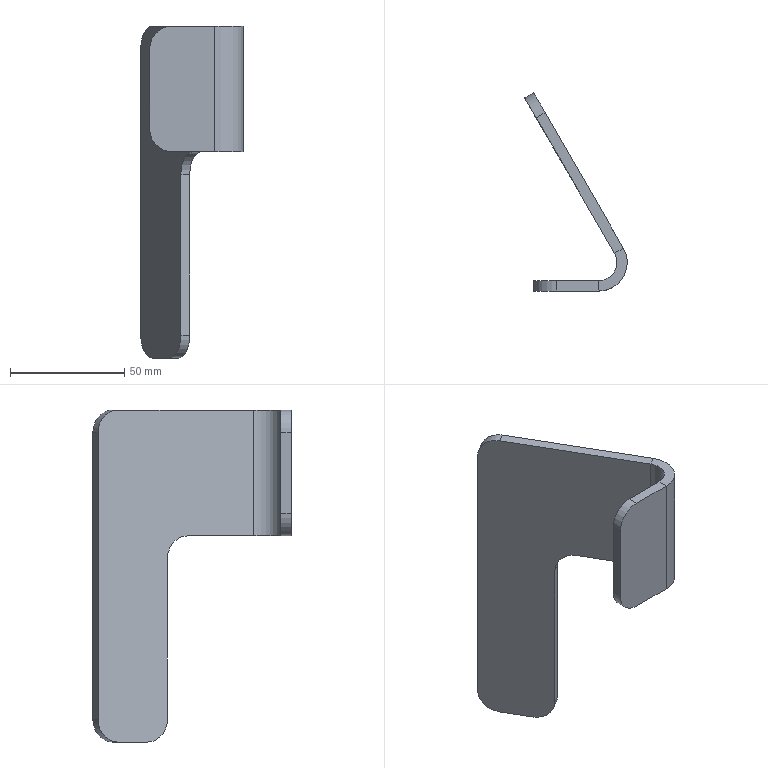Part | SolidWorks | features Fillet 1, FlatPattern 1, ICE 1, SMBaseFlange 1, SheetMetal 1 | 1 solid | 22 faces | box 44.746 x 86.603 x 145 mm | volume 45510 mm3 | plane 14 | cylinder 8 | commonest cylinder face diameters 20 x6 16 x1 25 x1
STEP:
#1=CARTESIAN_POINT('',(-40.,0.,17.5));
#2=VERTEX_POINT('',#1);
#3=CARTESIAN_POINT('',(-21.651,0.,17.5));
#4=VERTEX_POINT('',#3);
#5=CARTESIAN_POINT('',(0.,0.,17.5));
#6=DIRECTION('',(1.,0.,0.));
#7=VECTOR('',#6,1000.);
#8=LINE('',#5,#7);
#9=EDGE_CURVE('',#2,#4,#8,.T.);
#10=ORIENTED_EDGE('',*,*,#9,.F.);
#11=CARTESIAN_POINT('',(-40.,4.5,17.5));
#12=VERTEX_POINT('',#11);
#13=CARTESIAN_POINT('',(-40.,4.5,17.5));
#14=DIRECTION('',(0.,1.,0.));
#15=VECTOR('',#14,1000.);
#16=LINE('',#13,#15);
#17=EDGE_CURVE('',#2,#12,#16,.T.);
#18=ORIENTED_EDGE('',*,*,#17,.T.);
#19=CARTESIAN_POINT('',(-21.651,4.5,17.5));
#20=VERTEX_POINT('',#19);
#21=CARTESIAN_POINT('',(0.,4.5,17.5));
#22=DIRECTION('',(1.,0.,0.));
#23=VECTOR('',#22,1000.);
#24=LINE('',#21,#23);
#25=EDGE_CURVE('',#12,#20,#24,.T.);
#26=ORIENTED_EDGE('',*,*,#25,.T.);
#27=CARTESIAN_POINT('',(-21.651,4.5,17.5));
#28=DIRECTION('',(0.,-1.,0.));
#29=VECTOR('',#28,1000.);
#30=LINE('',#27,#29);
#31=EDGE_CURVE('',#20,#4,#30,.T.);
#32=ORIENTED_EDGE('',*,*,#31,.T.);
#33=EDGE_LOOP('',(#10,#18,#26,#32));
#34=FACE_OUTER_BOUND('',#33,.T.);
#35=CARTESIAN_POINT('',(-67.923,24.293,17.5));
#36=DIRECTION('',(0.,0.,1.));
#37=DIRECTION('',(0.,-1.,0.));
#38=AXIS2_PLACEMENT_3D('',#35,#36,#37);
#39=PLANE('',#38);
#40=ADVANCED_FACE('',(#34),#39,.F.);
#41=CARTESIAN_POINT('',(-27.5,47.631,17.5));
#42=VERTEX_POINT('',#41);
#43=CARTESIAN_POINT('',(-10.825,18.75,17.5));
#44=VERTEX_POINT('',#43);
#45=CARTESIAN_POINT('',(-27.5,47.631,17.5));
#46=DIRECTION('',(0.5,-0.866,0.));
#47=VECTOR('',#46,1000.);
#48=LINE('',#45,#47);
#49=EDGE_CURVE('',#42,#44,#48,.T.);
#50=ORIENTED_EDGE('',*,*,#49,.T.);
#51=CARTESIAN_POINT('',(-14.722,16.5,17.5));
#52=VERTEX_POINT('',#51);
#53=CARTESIAN_POINT('',(-10.825,18.75,17.5));
#54=DIRECTION('',(-0.866,-0.5,0.));
#55=VECTOR('',#54,1000.);
#56=LINE('',#53,#55);
#57=EDGE_CURVE('',#44,#52,#56,.T.);
#58=ORIENTED_EDGE('',*,*,#57,.T.);
#59=CARTESIAN_POINT('',(-31.397,45.381,17.5));
#60=VERTEX_POINT('',#59);
#61=CARTESIAN_POINT('',(-3.897,-2.25,17.5));
#62=DIRECTION('',(-0.5,0.866,0.));
#63=VECTOR('',#62,1000.);
#64=LINE('',#61,#63);
#65=EDGE_CURVE('',#52,#60,#64,.T.);
#66=ORIENTED_EDGE('',*,*,#65,.T.);
#67=CARTESIAN_POINT('',(-67.923,24.293,17.5));
#68=DIRECTION('',(0.866,0.5,0.));
#69=VECTOR('',#68,1000.);
#70=LINE('',#67,#69);
#71=EDGE_CURVE('',#60,#42,#70,.T.);
#72=ORIENTED_EDGE('',*,*,#71,.T.);
#73=EDGE_LOOP('',(#50,#58,#66,#72));
#74=FACE_OUTER_BOUND('',#73,.T.);
#75=CARTESIAN_POINT('',(-67.923,24.293,17.5));
#76=DIRECTION('',(0.,0.,1.));
#77=DIRECTION('',(0.,-1.,0.));
#78=AXIS2_PLACEMENT_3D('',#75,#76,#77);
#79=PLANE('',#78);
#80=ADVANCED_FACE('',(#74),#79,.F.);
#81=CARTESIAN_POINT('',(-21.651,0.,72.5));
#82=VERTEX_POINT('',#81);
#83=CARTESIAN_POINT('',(-21.651,4.5,72.5));
#84=VERTEX_POINT('',#83);
#85=CARTESIAN_POINT('',(-21.651,0.,72.5));
#86=DIRECTION('',(0.,1.,0.));
#87=VECTOR('',#86,1000.);
#88=LINE('',#85,#87);
#89=EDGE_CURVE('',#82,#84,#88,.T.);
#90=ORIENTED_EDGE('',*,*,#89,.F.);
#91=CARTESIAN_POINT('',(-10.825,18.75,72.5));
#92=VERTEX_POINT('',#91);
#93=CARTESIAN_POINT('',(-21.651,12.5,72.5));
#94=DIRECTION('',(0.,0.,1.));
#95=DIRECTION('',(-1.,0.,0.));
#96=AXIS2_PLACEMENT_3D('',#93,#94,#95);
#97=CIRCLE('',#96,12.5);
#98=EDGE_CURVE('',#82,#92,#97,.T.);
#99=ORIENTED_EDGE('',*,*,#98,.T.);
#100=CARTESIAN_POINT('',(-14.722,16.5,72.5));
#101=VERTEX_POINT('',#100);
#102=CARTESIAN_POINT('',(-14.722,16.5,72.5));
#103=DIRECTION('',(0.866,0.5,0.));
#104=VECTOR('',#103,1000.);
#105=LINE('',#102,#104);
#106=EDGE_CURVE('',#101,#92,#105,.T.);
#107=ORIENTED_EDGE('',*,*,#106,.F.);
#108=CARTESIAN_POINT('',(-21.651,12.5,72.5));
#109=DIRECTION('',(0.,0.,1.));
#110=DIRECTION('',(1.,0.,0.));
#111=AXIS2_PLACEMENT_3D('',#108,#109,#110);
#112=CIRCLE('',#111,8.);
#113=EDGE_CURVE('',#84,#101,#112,.T.);
#114=ORIENTED_EDGE('',*,*,#113,.F.);
#115=EDGE_LOOP('',(#90,#99,#107,#114));
#116=FACE_OUTER_BOUND('',#115,.T.);
#117=CARTESIAN_POINT('',(-21.651,0.,72.5));
#118=DIRECTION('',(0.,0.,1.));
#119=DIRECTION('',(1.,0.,0.));
#120=AXIS2_PLACEMENT_3D('',#117,#118,#119);
#121=PLANE('',#120);
#122=ADVANCED_FACE('',(#116),#121,.T.);
#123=CARTESIAN_POINT('',(-40.,4.5,72.5));
#124=VERTEX_POINT('',#123);
#125=CARTESIAN_POINT('',(0.,4.5,72.5));
#126=DIRECTION('',(1.,0.,0.));
#127=VECTOR('',#126,1000.);
#128=LINE('',#125,#127);
#129=EDGE_CURVE('',#124,#84,#128,.T.);
#130=ORIENTED_EDGE('',*,*,#129,.F.);
#131=CARTESIAN_POINT('',(-40.,0.,72.5));
#132=VERTEX_POINT('',#131);
#133=CARTESIAN_POINT('',(-40.,16.5,72.5));
#134=DIRECTION('',(0.,-1.,0.));
#135=VECTOR('',#134,1000.);
#136=LINE('',#133,#135);
#137=EDGE_CURVE('',#124,#132,#136,.T.);
#138=ORIENTED_EDGE('',*,*,#137,.T.);
#139=CARTESIAN_POINT('',(0.,0.,72.5));
#140=DIRECTION('',(1.,0.,0.));
#141=VECTOR('',#140,1000.);
#142=LINE('',#139,#141);
#143=EDGE_CURVE('',#132,#82,#142,.T.);
#144=ORIENTED_EDGE('',*,*,#143,.T.);
#145=ORIENTED_EDGE('',*,*,#89,.T.);
#146=EDGE_LOOP('',(#130,#138,#144,#145));
#147=FACE_OUTER_BOUND('',#146,.T.);
#148=CARTESIAN_POINT('',(-14.722,16.5,72.5));
#149=DIRECTION('',(0.,0.,1.));
#150=DIRECTION('',(1.,0.,0.));
#151=AXIS2_PLACEMENT_3D('',#148,#149,#150);
#152=PLANE('',#151);
#153=ADVANCED_FACE('',(#147),#152,.T.);
#154=CARTESIAN_POINT('',(-37.5,64.952,-72.5));
#155=VERTEX_POINT('',#154);
#156=CARTESIAN_POINT('',(-45.,77.942,-72.5));
#157=VERTEX_POINT('',#156);
#158=CARTESIAN_POINT('',(0.,0.,-72.5));
#159=DIRECTION('',(-0.5,0.866,0.));
#160=VECTOR('',#159,1000.);
#161=LINE('',#158,#160);
#162=EDGE_CURVE('',#155,#157,#161,.T.);
#163=ORIENTED_EDGE('',*,*,#162,.F.);
#164=CARTESIAN_POINT('',(-41.397,62.702,-72.5));
#165=VERTEX_POINT('',#164);
#166=CARTESIAN_POINT('',(-41.397,62.702,-72.5));
#167=DIRECTION('',(-0.866,-0.5,0.));
#168=VECTOR('',#167,1000.);
#169=LINE('',#166,#168);
#170=EDGE_CURVE('',#155,#165,#169,.T.);
#171=ORIENTED_EDGE('',*,*,#170,.T.);
#172=CARTESIAN_POINT('',(-48.897,75.692,-72.5));
#173=VERTEX_POINT('',#172);
#174=CARTESIAN_POINT('',(-3.897,-2.25,-72.5));
#175=DIRECTION('',(-0.5,0.866,0.));
#176=VECTOR('',#175,1000.);
#177=LINE('',#174,#176);
#178=EDGE_CURVE('',#165,#173,#177,.T.);
#179=ORIENTED_EDGE('',*,*,#178,.T.);
#180=CARTESIAN_POINT('',(-59.289,69.692,-72.5));
#181=DIRECTION('',(0.866,0.5,0.));
#182=VECTOR('',#181,1000.);
#183=LINE('',#180,#182);
#184=EDGE_CURVE('',#173,#157,#183,.T.);
#185=ORIENTED_EDGE('',*,*,#184,.T.);
#186=EDGE_LOOP('',(#163,#171,#179,#185));
#187=FACE_OUTER_BOUND('',#186,.T.);
#188=CARTESIAN_POINT('',(-21.651,4.5,-72.5));
#189=DIRECTION('',(0.,0.,-1.));
#190=DIRECTION('',(-1.,0.,0.));
#191=AXIS2_PLACEMENT_3D('',#188,#189,#190);
#192=PLANE('',#191);
#193=ADVANCED_FACE('',(#187),#192,.T.);
#194=CARTESIAN_POINT('',(-32.5,56.292,-62.5));
#195=VERTEX_POINT('',#194);
#196=CARTESIAN_POINT('',(-32.5,56.292,7.5));
#197=VERTEX_POINT('',#196);
#198=CARTESIAN_POINT('',(-32.5,56.292,-72.5));
#199=DIRECTION('',(0.,0.,1.));
#200=VECTOR('',#199,1000.);
#201=LINE('',#198,#200);
#202=EDGE_CURVE('',#195,#197,#201,.T.);
#203=ORIENTED_EDGE('',*,*,#202,.F.);
#204=CARTESIAN_POINT('',(-37.5,64.952,-62.5));
#205=DIRECTION('',(0.866,0.5,0.));
#206=DIRECTION('',(0.5,-0.866,0.));
#207=AXIS2_PLACEMENT_3D('',#204,#205,#206);
#208=CIRCLE('',#207,10.);
#209=EDGE_CURVE('',#195,#155,#208,.T.);
#210=ORIENTED_EDGE('',*,*,#209,.T.);
#211=ORIENTED_EDGE('',*,*,#162,.T.);
#212=CARTESIAN_POINT('',(-50.,86.603,-62.5));
#213=VERTEX_POINT('',#212);
#214=CARTESIAN_POINT('',(-45.,77.942,-62.5));
#215=DIRECTION('',(0.866,0.5,0.));
#216=DIRECTION('',(0.5,-0.866,0.));
#217=AXIS2_PLACEMENT_3D('',#214,#215,#216);
#218=CIRCLE('',#217,10.);
#219=EDGE_CURVE('',#157,#213,#218,.T.);
#220=ORIENTED_EDGE('',*,*,#219,.T.);
#221=CARTESIAN_POINT('',(-50.,86.603,62.5));
#222=VERTEX_POINT('',#221);
#223=CARTESIAN_POINT('',(-50.,86.603,72.5));
#224=DIRECTION('',(0.,0.,-1.));
#225=VECTOR('',#224,1000.);
#226=LINE('',#223,#225);
#227=EDGE_CURVE('',#222,#213,#226,.T.);
#228=ORIENTED_EDGE('',*,*,#227,.F.);
#229=CARTESIAN_POINT('',(-45.,77.942,72.5));
#230=VERTEX_POINT('',#229);
#231=CARTESIAN_POINT('',(-45.,77.942,62.5));
#232=DIRECTION('',(0.866,0.5,0.));
#233=DIRECTION('',(0.5,-0.866,0.));
#234=AXIS2_PLACEMENT_3D('',#231,#232,#233);
#235=CIRCLE('',#234,10.);
#236=EDGE_CURVE('',#222,#230,#235,.T.);
#237=ORIENTED_EDGE('',*,*,#236,.T.);
#238=CARTESIAN_POINT('',(0.,0.,72.5));
#239=DIRECTION('',(-0.5,0.866,0.));
#240=VECTOR('',#239,1000.);
#241=LINE('',#238,#240);
#242=EDGE_CURVE('',#92,#230,#241,.T.);
#243=ORIENTED_EDGE('',*,*,#242,.F.);
#244=CARTESIAN_POINT('',(-10.825,18.75,72.5));
#245=DIRECTION('',(0.,0.,-1.));
#246=VECTOR('',#245,1000.);
#247=LINE('',#244,#246);
#248=EDGE_CURVE('',#92,#44,#247,.T.);
#249=ORIENTED_EDGE('',*,*,#248,.T.);
#250=ORIENTED_EDGE('',*,*,#49,.F.);
#251=CARTESIAN_POINT('',(-27.5,47.631,7.5));
#252=DIRECTION('',(0.866,0.5,0.));
#253=DIRECTION('',(-0.5,0.866,0.));
#254=AXIS2_PLACEMENT_3D('',#251,#252,#253);
#255=CIRCLE('',#254,10.);
#256=EDGE_CURVE('',#197,#42,#255,.T.);
#257=ORIENTED_EDGE('',*,*,#256,.F.);
#258=EDGE_LOOP('',(#203,#210,#211,#220,#228,#237,#243,#249,#250,#257));
#259=FACE_OUTER_BOUND('',#258,.T.);
#260=CARTESIAN_POINT('',(0.,0.,72.5));
#261=DIRECTION('',(-0.866,-0.5,0.));
#262=DIRECTION('',(0.5,-0.866,0.));
#263=AXIS2_PLACEMENT_3D('',#260,#261,#262);
#264=PLANE('',#263);
#265=ADVANCED_FACE('',(#259),#264,.F.);
#266=ORIENTED_EDGE('',*,*,#227,.T.);
#267=CARTESIAN_POINT('',(-53.897,84.353,-62.5));
#268=VERTEX_POINT('',#267);
#269=CARTESIAN_POINT('',(-53.897,84.353,-62.5));
#270=DIRECTION('',(-0.866,-0.5,0.));
#271=VECTOR('',#270,1000.);
#272=LINE('',#269,#271);
#273=EDGE_CURVE('',#213,#268,#272,.T.);
#274=ORIENTED_EDGE('',*,*,#273,.T.);
#275=CARTESIAN_POINT('',(-53.897,84.353,62.5));
#276=VERTEX_POINT('',#275);
#277=CARTESIAN_POINT('',(-53.897,84.353,72.5));
#278=DIRECTION('',(0.,0.,-1.));
#279=VECTOR('',#278,1000.);
#280=LINE('',#277,#279);
#281=EDGE_CURVE('',#276,#268,#280,.T.);
#282=ORIENTED_EDGE('',*,*,#281,.F.);
#283=CARTESIAN_POINT('',(-53.897,84.353,62.5));
#284=DIRECTION('',(0.866,0.5,0.));
#285=VECTOR('',#284,1000.);
#286=LINE('',#283,#285);
#287=EDGE_CURVE('',#276,#222,#286,.T.);
#288=ORIENTED_EDGE('',*,*,#287,.T.);
#289=EDGE_LOOP('',(#266,#274,#282,#288));
#290=FACE_OUTER_BOUND('',#289,.T.);
#291=CARTESIAN_POINT('',(-53.897,84.353,72.5));
#292=DIRECTION('',(-0.5,0.866,0.));
#293=DIRECTION('',(-0.866,-0.5,0.));
#294=AXIS2_PLACEMENT_3D('',#291,#292,#293);
#295=PLANE('',#294);
#296=ADVANCED_FACE('',(#290),#295,.T.);
#297=ORIENTED_EDGE('',*,*,#178,.F.);
#298=CARTESIAN_POINT('',(-36.397,54.042,-62.5));
#299=VERTEX_POINT('',#298);
#300=CARTESIAN_POINT('',(-41.397,62.702,-62.5));
#301=DIRECTION('',(-0.866,-0.5,0.));
#302=DIRECTION('',(0.5,-0.866,0.));
#303=AXIS2_PLACEMENT_3D('',#300,#301,#302);
#304=CIRCLE('',#303,10.);
#305=EDGE_CURVE('',#165,#299,#304,.T.);
#306=ORIENTED_EDGE('',*,*,#305,.T.);
#307=CARTESIAN_POINT('',(-36.397,54.042,7.5));
#308=VERTEX_POINT('',#307);
#309=CARTESIAN_POINT('',(-36.397,54.042,72.5));
#310=DIRECTION('',(0.,0.,-1.));
#311=VECTOR('',#310,1000.);
#312=LINE('',#309,#311);
#313=EDGE_CURVE('',#308,#299,#312,.T.);
#314=ORIENTED_EDGE('',*,*,#313,.F.);
#315=CARTESIAN_POINT('',(-31.397,45.381,7.5));
#316=DIRECTION('',(-0.866,-0.5,0.));
#317=DIRECTION('',(0.5,-0.866,0.));
#318=AXIS2_PLACEMENT_3D('',#315,#316,#317);
#319=CIRCLE('',#318,10.);
#320=EDGE_CURVE('',#60,#308,#319,.T.);
#321=ORIENTED_EDGE('',*,*,#320,.F.);
#322=ORIENTED_EDGE('',*,*,#65,.F.);
#323=CARTESIAN_POINT('',(-14.722,16.5,72.5));
#324=DIRECTION('',(0.,0.,-1.));
#325=VECTOR('',#324,1000.);
#326=LINE('',#323,#325);
#327=EDGE_CURVE('',#101,#52,#326,.T.);
#328=ORIENTED_EDGE('',*,*,#327,.F.);
#329=CARTESIAN_POINT('',(-48.897,75.692,72.5));
#330=VERTEX_POINT('',#329);
#331=CARTESIAN_POINT('',(-3.897,-2.25,72.5));
#332=DIRECTION('',(-0.5,0.866,0.));
#333=VECTOR('',#332,1000.);
#334=LINE('',#331,#333);
#335=EDGE_CURVE('',#101,#330,#334,.T.);
#336=ORIENTED_EDGE('',*,*,#335,.T.);
#337=CARTESIAN_POINT('',(-48.897,75.692,62.5));
#338=DIRECTION('',(-0.866,-0.5,0.));
#339=DIRECTION('',(0.5,-0.866,0.));
#340=AXIS2_PLACEMENT_3D('',#337,#338,#339);
#341=CIRCLE('',#340,10.);
#342=EDGE_CURVE('',#330,#276,#341,.T.);
#343=ORIENTED_EDGE('',*,*,#342,.T.);
#344=ORIENTED_EDGE('',*,*,#281,.T.);
#345=CARTESIAN_POINT('',(-48.897,75.692,-62.5));
#346=DIRECTION('',(-0.866,-0.5,0.));
#347=DIRECTION('',(0.5,-0.866,0.));
#348=AXIS2_PLACEMENT_3D('',#345,#346,#347);
#349=CIRCLE('',#348,10.);
#350=EDGE_CURVE('',#268,#173,#349,.T.);
#351=ORIENTED_EDGE('',*,*,#350,.T.);
#352=EDGE_LOOP('',(#297,#306,#314,#321,#322,#328,#336,#343,#344,#351));
#353=FACE_OUTER_BOUND('',#352,.T.);
#354=CARTESIAN_POINT('',(-3.897,-2.25,72.5));
#355=DIRECTION('',(-0.866,-0.5,0.));
#356=DIRECTION('',(0.5,-0.866,0.));
#357=AXIS2_PLACEMENT_3D('',#354,#355,#356);
#358=PLANE('',#357);
#359=ADVANCED_FACE('',(#353),#358,.T.);
#360=CARTESIAN_POINT('',(-21.651,12.5,17.5));
#361=DIRECTION('',(0.,0.,1.));
#362=DIRECTION('',(0.,-1.,0.));
#363=AXIS2_PLACEMENT_3D('',#360,#361,#362);
#364=CIRCLE('',#363,8.);
#365=EDGE_CURVE('',#20,#52,#364,.T.);
#366=ORIENTED_EDGE('',*,*,#365,.F.);
#367=CARTESIAN_POINT('',(-21.651,4.5,72.5));
#368=DIRECTION('',(0.,0.,-1.));
#369=VECTOR('',#368,1000.);
#370=LINE('',#367,#369);
#371=EDGE_CURVE('',#84,#20,#370,.T.);
#372=ORIENTED_EDGE('',*,*,#371,.F.);
#373=ORIENTED_EDGE('',*,*,#113,.T.);
#374=ORIENTED_EDGE('',*,*,#327,.T.);
#375=EDGE_LOOP('',(#366,#372,#373,#374));
#376=FACE_OUTER_BOUND('',#375,.T.);
#377=CARTESIAN_POINT('',(-21.651,12.5,72.5));
#378=DIRECTION('',(0.,0.,-1.));
#379=DIRECTION('',(-1.,0.,0.));
#380=AXIS2_PLACEMENT_3D('',#377,#378,#379);
#381=CYLINDRICAL_SURFACE('',#380,8.);
#382=ADVANCED_FACE('',(#376),#381,.F.);
#383=ORIENTED_EDGE('',*,*,#25,.F.);
#384=CARTESIAN_POINT('',(-50.,4.5,27.5));
#385=VERTEX_POINT('',#384);
#386=CARTESIAN_POINT('',(-40.,4.5,27.5));
#387=DIRECTION('',(0.,1.,0.));
#388=DIRECTION('',(0.,0.,1.));
#389=AXIS2_PLACEMENT_3D('',#386,#387,#388);
#390=CIRCLE('',#389,10.);
#391=EDGE_CURVE('',#12,#385,#390,.T.);
#392=ORIENTED_EDGE('',*,*,#391,.T.);
#393=CARTESIAN_POINT('',(-50.,4.5,62.5));
#394=VERTEX_POINT('',#393);
#395=CARTESIAN_POINT('',(-50.,4.5,72.5));
#396=DIRECTION('',(0.,0.,-1.));
#397=VECTOR('',#396,1000.);
#398=LINE('',#395,#397);
#399=EDGE_CURVE('',#394,#385,#398,.T.);
#400=ORIENTED_EDGE('',*,*,#399,.F.);
#401=CARTESIAN_POINT('',(-40.,4.5,62.5));
#402=DIRECTION('',(0.,1.,0.));
#403=DIRECTION('',(0.,0.,1.));
#404=AXIS2_PLACEMENT_3D('',#401,#402,#403);
#405=CIRCLE('',#404,10.);
#406=EDGE_CURVE('',#394,#124,#405,.T.);
#407=ORIENTED_EDGE('',*,*,#406,.T.);
#408=ORIENTED_EDGE('',*,*,#129,.T.);
#409=ORIENTED_EDGE('',*,*,#371,.T.);
#410=EDGE_LOOP('',(#383,#392,#400,#407,#408,#409));
#411=FACE_OUTER_BOUND('',#410,.T.);
#412=CARTESIAN_POINT('',(0.,4.5,72.5));
#413=DIRECTION('',(0.,1.,0.));
#414=DIRECTION('',(0.,0.,1.));
#415=AXIS2_PLACEMENT_3D('',#412,#413,#414);
#416=PLANE('',#415);
#417=ADVANCED_FACE('',(#411),#416,.T.);
#418=ORIENTED_EDGE('',*,*,#399,.T.);
#419=CARTESIAN_POINT('',(-50.,0.,27.5));
#420=VERTEX_POINT('',#419);
#421=CARTESIAN_POINT('',(-50.,0.,27.5));
#422=DIRECTION('',(0.,-1.,0.));
#423=VECTOR('',#422,1000.);
#424=LINE('',#421,#423);
#425=EDGE_CURVE('',#385,#420,#424,.T.);
#426=ORIENTED_EDGE('',*,*,#425,.T.);
#427=CARTESIAN_POINT('',(-50.,0.,62.5));
#428=VERTEX_POINT('',#427);
#429=CARTESIAN_POINT('',(-50.,0.,72.5));
#430=DIRECTION('',(0.,0.,-1.));
#431=VECTOR('',#430,1000.);
#432=LINE('',#429,#431);
#433=EDGE_CURVE('',#428,#420,#432,.T.);
#434=ORIENTED_EDGE('',*,*,#433,.F.);
#435=CARTESIAN_POINT('',(-50.,0.,62.5));
#436=DIRECTION('',(0.,1.,0.));
#437=VECTOR('',#436,1000.);
#438=LINE('',#435,#437);
#439=EDGE_CURVE('',#428,#394,#438,.T.);
#440=ORIENTED_EDGE('',*,*,#439,.T.);
#441=EDGE_LOOP('',(#418,#426,#434,#440));
#442=FACE_OUTER_BOUND('',#441,.T.);
#443=CARTESIAN_POINT('',(-50.,0.,72.5));
#444=DIRECTION('',(-1.,0.,0.));
#445=DIRECTION('',(0.,0.,1.));
#446=AXIS2_PLACEMENT_3D('',#443,#444,#445);
#447=PLANE('',#446);
#448=ADVANCED_FACE('',(#442),#447,.T.);
#449=ORIENTED_EDGE('',*,*,#433,.T.);
#450=CARTESIAN_POINT('',(-40.,0.,27.5));
#451=DIRECTION('',(0.,-1.,0.));
#452=DIRECTION('',(0.,0.,1.));
#453=AXIS2_PLACEMENT_3D('',#450,#451,#452);
#454=CIRCLE('',#453,10.);
#455=EDGE_CURVE('',#420,#2,#454,.T.);
#456=ORIENTED_EDGE('',*,*,#455,.T.);
#457=ORIENTED_EDGE('',*,*,#9,.T.);
#458=CARTESIAN_POINT('',(-21.651,0.,72.5));
#459=DIRECTION('',(0.,0.,-1.));
#460=VECTOR('',#459,1000.);
#461=LINE('',#458,#460);
#462=EDGE_CURVE('',#82,#4,#461,.T.);
#463=ORIENTED_EDGE('',*,*,#462,.F.);
#464=ORIENTED_EDGE('',*,*,#143,.F.);
#465=CARTESIAN_POINT('',(-40.,0.,62.5));
#466=DIRECTION('',(0.,-1.,0.));
#467=DIRECTION('',(0.,0.,1.));
#468=AXIS2_PLACEMENT_3D('',#465,#466,#467);
#469=CIRCLE('',#468,10.);
#470=EDGE_CURVE('',#132,#428,#469,.T.);
#471=ORIENTED_EDGE('',*,*,#470,.T.);
#472=EDGE_LOOP('',(#449,#456,#457,#463,#464,#471));
#473=FACE_OUTER_BOUND('',#472,.T.);
#474=CARTESIAN_POINT('',(0.,0.,72.5));
#475=DIRECTION('',(0.,1.,0.));
#476=DIRECTION('',(0.,0.,1.));
#477=AXIS2_PLACEMENT_3D('',#474,#475,#476);
#478=PLANE('',#477);
#479=ADVANCED_FACE('',(#473),#478,.F.);
#480=ORIENTED_EDGE('',*,*,#462,.T.);
#481=CARTESIAN_POINT('',(-21.651,12.5,17.5));
#482=DIRECTION('',(0.,0.,1.));
#483=DIRECTION('',(0.,-1.,0.));
#484=AXIS2_PLACEMENT_3D('',#481,#482,#483);
#485=CIRCLE('',#484,12.5);
#486=EDGE_CURVE('',#4,#44,#485,.T.);
#487=ORIENTED_EDGE('',*,*,#486,.T.);
#488=ORIENTED_EDGE('',*,*,#248,.F.);
#489=ORIENTED_EDGE('',*,*,#98,.F.);
#490=EDGE_LOOP('',(#480,#487,#488,#489));
#491=FACE_OUTER_BOUND('',#490,.T.);
#492=CARTESIAN_POINT('',(-21.651,12.5,72.5));
#493=DIRECTION('',(0.,0.,-1.));
#494=DIRECTION('',(-1.,0.,0.));
#495=AXIS2_PLACEMENT_3D('',#492,#493,#494);
#496=CYLINDRICAL_SURFACE('',#495,12.5);
#497=ADVANCED_FACE('',(#491),#496,.T.);
#498=ORIENTED_EDGE('',*,*,#242,.T.);
#499=CARTESIAN_POINT('',(-55.825,71.692,72.5));
#500=DIRECTION('',(-0.866,-0.5,0.));
#501=VECTOR('',#500,1000.);
#502=LINE('',#499,#501);
#503=EDGE_CURVE('',#230,#330,#502,.T.);
#504=ORIENTED_EDGE('',*,*,#503,.T.);
#505=ORIENTED_EDGE('',*,*,#335,.F.);
#506=ORIENTED_EDGE('',*,*,#106,.T.);
#507=EDGE_LOOP('',(#498,#504,#505,#506));
#508=FACE_OUTER_BOUND('',#507,.T.);
#509=CARTESIAN_POINT('',(-21.651,12.5,72.5));
#510=DIRECTION('',(0.,0.,1.));
#511=DIRECTION('',(1.,0.,0.));
#512=AXIS2_PLACEMENT_3D('',#509,#510,#511);
#513=PLANE('',#512);
#514=ADVANCED_FACE('',(#508),#513,.T.);
#515=ORIENTED_EDGE('',*,*,#31,.F.);
#516=ORIENTED_EDGE('',*,*,#365,.T.);
#517=ORIENTED_EDGE('',*,*,#57,.F.);
#518=ORIENTED_EDGE('',*,*,#486,.F.);
#519=EDGE_LOOP('',(#515,#516,#517,#518));
#520=FACE_OUTER_BOUND('',#519,.T.);
#521=CARTESIAN_POINT('',(-67.923,24.293,17.5));
#522=DIRECTION('',(0.,0.,1.));
#523=DIRECTION('',(0.,-1.,0.));
#524=AXIS2_PLACEMENT_3D('',#521,#522,#523);
#525=PLANE('',#524);
#526=ADVANCED_FACE('',(#520),#525,.F.);
#527=ORIENTED_EDGE('',*,*,#320,.T.);
#528=CARTESIAN_POINT('',(-72.923,32.954,7.5));
#529=DIRECTION('',(0.866,0.5,0.));
#530=VECTOR('',#529,1000.);
#531=LINE('',#528,#530);
#532=EDGE_CURVE('',#308,#197,#531,.T.);
#533=ORIENTED_EDGE('',*,*,#532,.T.);
#534=ORIENTED_EDGE('',*,*,#256,.T.);
#535=ORIENTED_EDGE('',*,*,#71,.F.);
#536=EDGE_LOOP('',(#527,#533,#534,#535));
#537=FACE_OUTER_BOUND('',#536,.T.);
#538=CARTESIAN_POINT('',(-67.923,24.293,7.5));
#539=DIRECTION('',(0.866,0.5,0.));
#540=DIRECTION('',(-0.5,0.866,0.));
#541=AXIS2_PLACEMENT_3D('',#538,#539,#540);
#542=CYLINDRICAL_SURFACE('',#541,10.);
#543=ADVANCED_FACE('',(#537),#542,.F.);
#544=ORIENTED_EDGE('',*,*,#313,.T.);
#545=CARTESIAN_POINT('',(-32.5,56.292,-62.5));
#546=DIRECTION('',(0.866,0.5,0.));
#547=VECTOR('',#546,1000.);
#548=LINE('',#545,#547);
#549=EDGE_CURVE('',#299,#195,#548,.T.);
#550=ORIENTED_EDGE('',*,*,#549,.T.);
#551=ORIENTED_EDGE('',*,*,#202,.T.);
#552=ORIENTED_EDGE('',*,*,#532,.F.);
#553=EDGE_LOOP('',(#544,#550,#551,#552));
#554=FACE_OUTER_BOUND('',#553,.T.);
#555=CARTESIAN_POINT('',(-72.923,32.954,-72.5));
#556=DIRECTION('',(-0.5,0.866,0.));
#557=DIRECTION('',(-0.866,-0.5,0.));
#558=AXIS2_PLACEMENT_3D('',#555,#556,#557);
#559=PLANE('',#558);
#560=ADVANCED_FACE('',(#554),#559,.F.);
#561=ORIENTED_EDGE('',*,*,#305,.F.);
#562=ORIENTED_EDGE('',*,*,#170,.F.);
#563=ORIENTED_EDGE('',*,*,#209,.F.);
#564=ORIENTED_EDGE('',*,*,#549,.F.);
#565=EDGE_LOOP('',(#561,#562,#563,#564));
#566=FACE_OUTER_BOUND('',#565,.T.);
#567=CARTESIAN_POINT('',(-77.923,41.614,-62.5));
#568=DIRECTION('',(-0.866,-0.5,0.));
#569=DIRECTION('',(0.5,-0.866,0.));
#570=AXIS2_PLACEMENT_3D('',#567,#568,#569);
#571=CYLINDRICAL_SURFACE('',#570,10.);
#572=ADVANCED_FACE('',(#566),#571,.T.);
#573=ORIENTED_EDGE('',*,*,#350,.F.);
#574=ORIENTED_EDGE('',*,*,#273,.F.);
#575=ORIENTED_EDGE('',*,*,#219,.F.);
#576=ORIENTED_EDGE('',*,*,#184,.F.);
#577=EDGE_LOOP('',(#573,#574,#575,#576));
#578=FACE_OUTER_BOUND('',#577,.T.);
#579=CARTESIAN_POINT('',(-59.289,69.692,-62.5));
#580=DIRECTION('',(0.866,0.5,0.));
#581=DIRECTION('',(-0.5,0.866,0.));
#582=AXIS2_PLACEMENT_3D('',#579,#580,#581);
#583=CYLINDRICAL_SURFACE('',#582,10.);
#584=ADVANCED_FACE('',(#578),#583,.T.);
#585=ORIENTED_EDGE('',*,*,#455,.F.);
#586=ORIENTED_EDGE('',*,*,#425,.F.);
#587=ORIENTED_EDGE('',*,*,#391,.F.);
#588=ORIENTED_EDGE('',*,*,#17,.F.);
#589=EDGE_LOOP('',(#585,#586,#587,#588));
#590=FACE_OUTER_BOUND('',#589,.T.);
#591=CARTESIAN_POINT('',(-40.,24.293,27.5));
#592=DIRECTION('',(0.,-1.,0.));
#593=DIRECTION('',(0.,0.,-1.));
#594=AXIS2_PLACEMENT_3D('',#591,#592,#593);
#595=CYLINDRICAL_SURFACE('',#594,10.);
#596=ADVANCED_FACE('',(#590),#595,.T.);
#597=ORIENTED_EDGE('',*,*,#470,.F.);
#598=ORIENTED_EDGE('',*,*,#137,.F.);
#599=ORIENTED_EDGE('',*,*,#406,.F.);
#600=ORIENTED_EDGE('',*,*,#439,.F.);
#601=EDGE_LOOP('',(#597,#598,#599,#600));
#602=FACE_OUTER_BOUND('',#601,.T.);
#603=CARTESIAN_POINT('',(-40.,0.,62.5));
#604=DIRECTION('',(0.,1.,0.));
#605=DIRECTION('',(0.,0.,1.));
#606=AXIS2_PLACEMENT_3D('',#603,#604,#605);
#607=CYLINDRICAL_SURFACE('',#606,10.);
#608=ADVANCED_FACE('',(#602),#607,.T.);
#609=ORIENTED_EDGE('',*,*,#342,.F.);
#610=ORIENTED_EDGE('',*,*,#503,.F.);
#611=ORIENTED_EDGE('',*,*,#236,.F.);
#612=ORIENTED_EDGE('',*,*,#287,.F.);
#613=EDGE_LOOP('',(#609,#610,#611,#612));
#614=FACE_OUTER_BOUND('',#613,.T.);
#615=CARTESIAN_POINT('',(-48.897,75.692,62.5));
#616=DIRECTION('',(0.866,0.5,0.));
#617=DIRECTION('',(-0.5,0.866,0.));
#618=AXIS2_PLACEMENT_3D('',#615,#616,#617);
#619=CYLINDRICAL_SURFACE('',#618,10.);
#620=ADVANCED_FACE('',(#614),#619,.T.);
#621=CLOSED_SHELL('',(#40,#80,#122,#153,#193,#265,#296,#359,#382,#417,#448,#479,#497,#514,#526,#543,#560,#572,#584,#596,#608,#620));
#622=MANIFOLD_SOLID_BREP('',#621);
#623=CARTESIAN_POINT('',(0.,0.,0.));
#624=DIRECTION('',(0.,0.,1.));
#625=DIRECTION('',(1.,0.,0.));
#626=AXIS2_PLACEMENT_3D('',#623,#624,#625);
#627=(LENGTH_UNIT()NAMED_UNIT(*)SI_UNIT(.MILLI.,.METRE.));
#628=UNCERTAINTY_MEASURE_WITH_UNIT(LENGTH_MEASURE(0.00001),#627,'','');
#629=(NAMED_UNIT(*)PLANE_ANGLE_UNIT()SI_UNIT($,.RADIAN.));
#630=(NAMED_UNIT(*)SI_UNIT($,.STERADIAN.)SOLID_ANGLE_UNIT());
#631=(GEOMETRIC_REPRESENTATION_CONTEXT(3)GLOBAL_UNCERTAINTY_ASSIGNED_CONTEXT((#628))GLOBAL_UNIT_ASSIGNED_CONTEXT((#627,#629,#630))REPRESENTATION_CONTEXT('',''));
#632=ADVANCED_BREP_SHAPE_REPRESENTATION('',(#622,#626),#631);